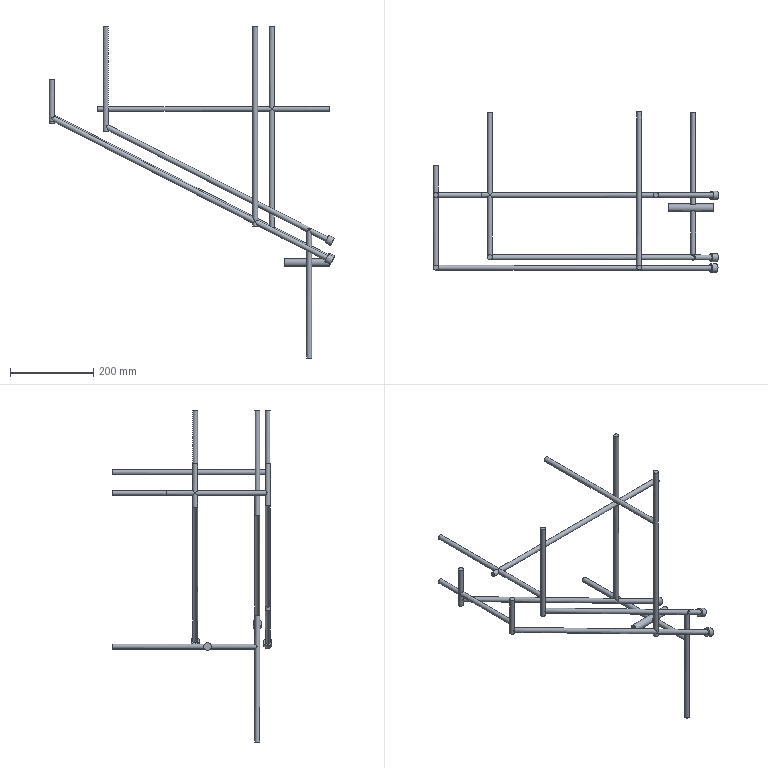Part | STEP file | solid 257 | 1 solid | 65 faces | box 687.344 x 385 x 800 mm | volume 676592 mm3 | plane 33 | cylinder 32 | commonest cylinder face diameters 12 x28 20 x3 18.5 x1